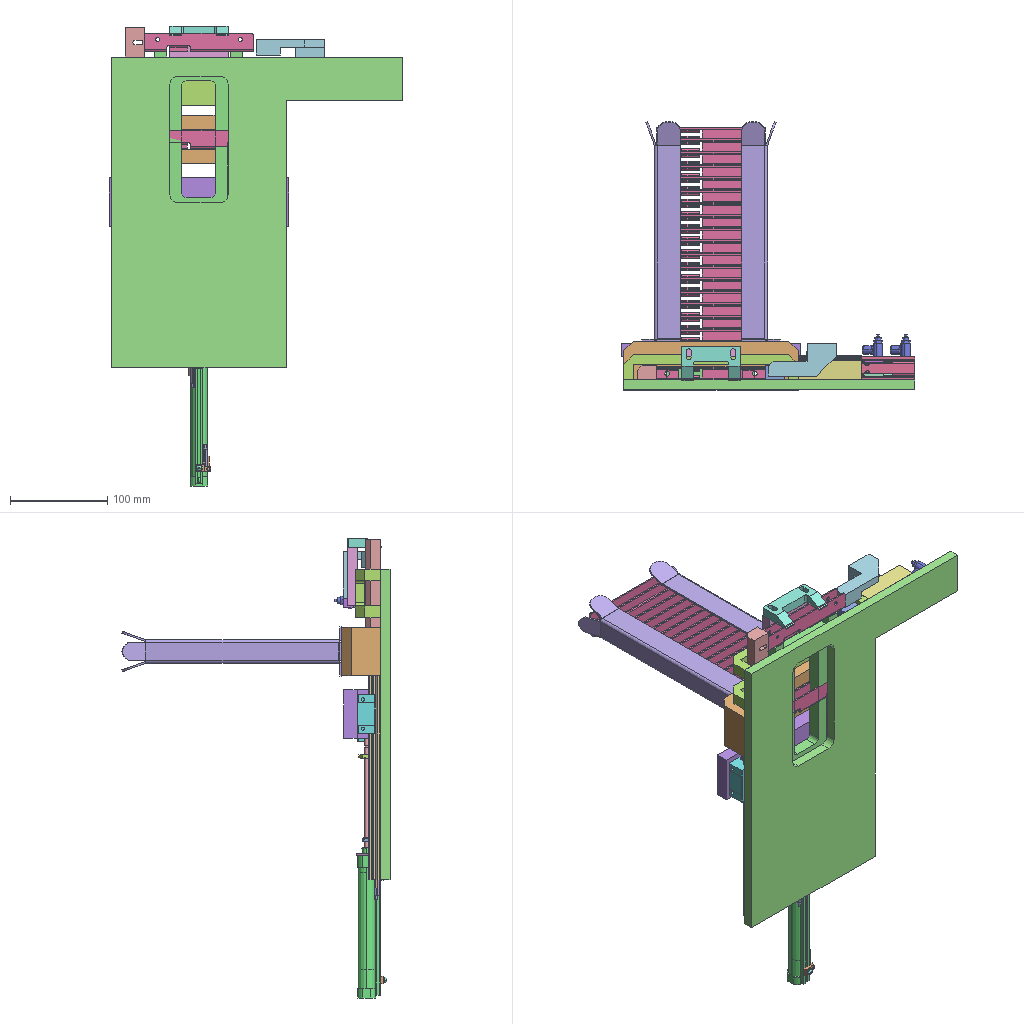Assembly | SolidWorks | 37 different items | 66 placed | box 303 x 276 x 474 mm
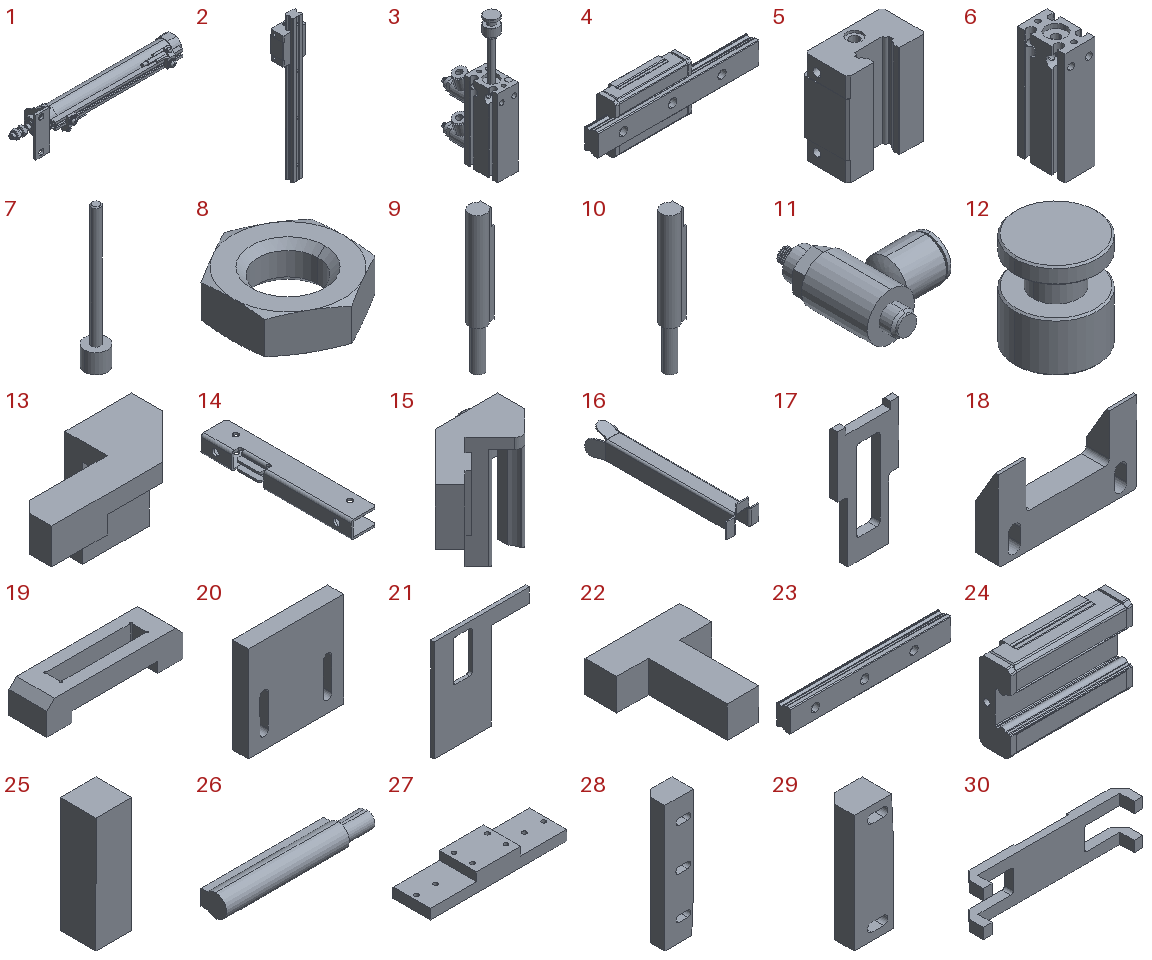Parts list (item | name | quantity | parent item | size | volume | features):
1 | (subassembly) | x1 | - | 175 x 31.65 x 42 mm | 27316 mm3 | -
2 | (subassembly) | x2 | - | 34 x 24 x 210 mm | 54732 mm3 | -
3 | (subassembly) | x1 | - | 16.622 x 46.7 x 96.543 mm | 20146 mm3 | -
4 | (subassembly) | x1 | - | 65 x 10 x 20 mm | 6401 mm3 | -
5 | - | x2 | in 2 | 34 x 19.5 x 40.1 mm | 21289 mm3 | features BaseBody 1
6 | - | x1 | in 3 | 15 x 24 x 56 mm | 13473 mm3 | features BaseBody 1
7 | - | x1 | in 3 | 10 x 10 x 62.6 mm | 1353 mm3 | features BaseBody 1
8 | - | x1 | in 3 | 6 x 6.928 x 2 mm | 44.043 mm3 | features BaseBody 1
9 | - | x1 | in 3 | 4.6 x 4 x 33.5 mm | 397.477 mm3 | features BaseBody 1
10 | - | x1 | in 3 | 4.6 x 4 x 33.5 mm | 397.477 mm3 | features BaseBody 1
11 | - | x2 | in 3 | 20.5 x 26.2 x 10 mm | 1922 mm3 | features BaseBody 1
12 | - | x1 | in 3 | 10 x 10 x 11.5 mm | 637.742 mm3 | features ICE 2, Chamfer 1, Extrusion 1, HoleWzd 1
13 | - | x1 | - | 70 x 34 x 48 mm | 23760 mm3 | features ICE 3, Chamfer 2, Extrusion 1
14 | - | x21 | - | 19 x 112 x 13 mm | 7436 mm3 | features BaseBody 1
15 | - | x2 | in 1 | 15.769 x 11.133 x 16 mm | 523.118 mm3 | features RefAxis 6, ICE 4, 3DProfileFeature 2, Extrusion 1, RevCut 1, Revolution 1
16 | - | x2 | - | 50.5 x 226.176 x 40 mm | 34108 mm3 | features EdgeFlange 3, Fillet 1, FlatPattern 1, SMBaseFlange 1, SheetMetal 1
17 | - | x1 | - | 90 x 12.5 x 180 mm | 108281 mm3 | features Fillet 3, Cut 2, Chamfer 1, Extrusion 1, ICE 1
18 | - | x1 | - | 60 x 10 x 35 mm | 11142 mm3 | features Chamfer 2, Cut 1, Extrusion 1, Fillet 1, ICE 1, MirrorPattern 1
19 | - | x1 | - | 180 x 50 x 40 mm | 216729 mm3 | features ICE 3, Chamfer 1, Cut 1, Extrusion 1
20 | - | x1 | - | 60 x 10 x 60 mm | 33382 mm3 | features Cut 1, Extrusion 1, MirrorPattern 1
21 | - | x1 | - | 300 x 10 x 320 mm | 552549 mm3 | features Cut 1, Extrusion 1, Fillet 1, ICE 1
22 | - | x1 | - | 30 x 35 x 10 mm | 5500 mm3 | features Extrusion 1, ICE 1
23 | - | x1 | in 4 | 65 x 5.5 x 9 mm | 2567 mm3 | features BaseBody 1, Cut 1, HoleWzd 1, ICE 1, LPattern 1
24 | - | x1 | in 4 | 30.8 x 8.5 x 20 mm | 3834 mm3 | features BaseBody 1
25 | - | x1 | - | 20 x 20 x 65 mm | 26000 mm3 | features Extrusion 1
26 | - | x2 | in 1 | 27 x 4.6 x 4 mm | 358.79 mm3 | features RefAxis 3, 3DProfileFeature 1, Extrusion 1, HoleWzd 1, ICE 1
27 | - | x1 | - | 185 x 50 x 25 mm | 153218 mm3 | features HoleWzd 2, Extrusion 1, ICE 1
28 | - | x1 | - | 20 x 15 x 90 mm | 22961 mm3 | features Cut 3, Chamfer 1, Extrusion 1, LPattern 1
29 | - | x1 | - | 20 x 15 x 60 mm | 15035 mm3 | features Cut 3, Chamfer 1, Extrusion 1, MirrorPattern 1
30 | - | x1 | - | 180 x 26 x 50 mm | 63357 mm3 | features Cut 2, Chamfer 1, Extrusion 1, Fillet 1, ICE 1, MirrorPattern 1
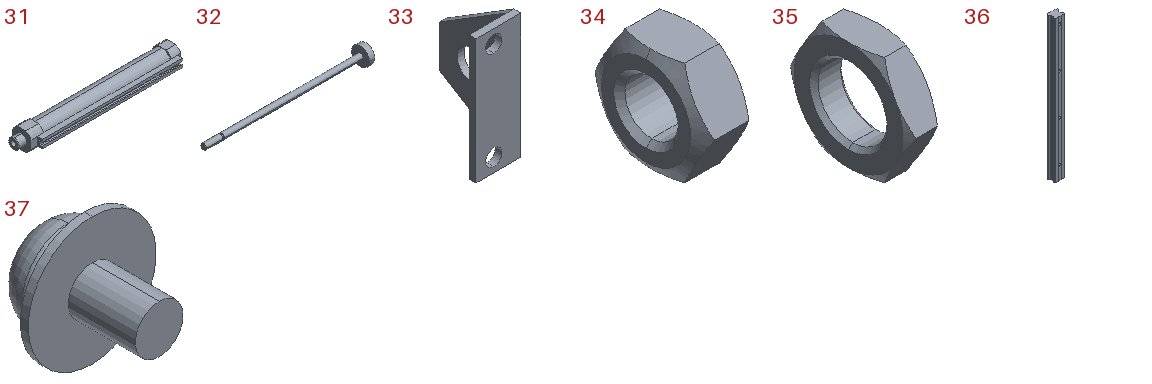31 | - | x1 | in 1 | 155 x 23.3 x 18.3 mm | 18210 mm3 | features RefAxis 21, 3DProfileFeature 7, ICE 4, HoleWzd 2, Revolution 2, LPattern 1, RevCut 1
32 | - | x1 | in 1 | 145.5 x 16 x 16 mm | 3753 mm3 | features RefAxis 9, 3DProfileFeature 3, Revolution 1
33 | - | x1 | in 1 | 15 x 25 x 42 mm | 2621 mm3 | features RefAxis 3, ICE 2, 3DProfileFeature 1, Extrusion 1, HoleWzd 1, LPattern 1
34 | - | x2 | in 1 | 4 x 9.238 x 8 mm | 156.615 mm3 | features RefAxis 6, 3DProfileFeature 2, RevCut 2, Extrusion 1
35 | - | x1 | in 1 | 4 x 16.166 x 14 mm | 414.657 mm3 | features RefAxis 6, 3DProfileFeature 2, RevCut 2, Extrusion 1
36 | - | x2 | in 2 | 15 x 12.5 x 210 mm | 33443 mm3 | features BaseBody 1, HoleWzd 1, ICE 1, LPattern 1
37 | - | x2 | in 1 | 8 x 7.7 x 8 mm | 119.911 mm3 | features RefAxis 6, 3DProfileFeature 2, Revolution 1
Mates (type | each side: item.copy, entity, surface, feature):
In the top assembly
Coincident | 28.1 face plane Boss-Extrude1 | 19.1 face plane Boss-Extrude1
Coincident | 30.1 face plane Cut-Extrude2 | 20.1 face plane Boss-Extrude1 | 2 times
Coincident | 20.1 face plane Boss-Extrude1 | 18.1 face plane Boss-Extrude1 | 2 times
Width | 20.1 face plane Boss-Extrude1 | 20.1 face plane Boss-Extrude1 | 18.1 face plane Boss-Extrude1 | 18.1 face plane Boss-Extrude1
Coincident | 19.1 face plane Boss-Extrude1 | 16.1 face plane Edge-Flange2
Coincident | 19.1 face plane Boss-Extrude1 | 16.2 face plane Edge-Flange2
Width | 19.1 face plane Cut-Extrude3 | 19.1 face plane Cut-Extrude3 | 17.1 face plane Boss-Extrude1 | 17.1 face plane Boss-Extrude1
Coincident | 19.1 face plane Boss-Extrude1 | 36.1 face plane Boss-Extrude1
Coincident | 19.1 face plane Boss-Extrude1 | 36.2 face plane Boss-Extrude1
Coincident | 16.1 face plane Edge-Flange1 | 16.2 face plane Edge-Flange1
Coincident | 17.1 face plane Boss-Extrude1 | 27.1 face plane Boss-Extrude1 | 2 times
Coincident | 5.1 face plane Import1 | 27.1 face plane Cut-Extrude1
Width | 5.1 face plane Import1 | 5.2 face plane Import1 | 27.1 face plane Boss-Extrude1 | 27.1 face plane Boss-Extrude1
Coincident | 21.1 face plane Boss-Extrude1 | 28.1 face plane Boss-Extrude1
DistanceDim | 21.1 face plane Boss-Extrude1 | 28.1 face plane Boss-Extrude1
Coincident | 21.1 face plane Boss-Extrude1 | 29.1 face plane Boss-Extrude1 | 2 times
Coincident | 21.1 face plane Boss-Extrude1 | 30.1 face plane Boss-Extrude2
Width | 21.1 face plane Boss-Extrude1 | 21.1 face plane Boss-Extrude1 | 30.1 face plane Boss-Extrude1 | 30.1 face plane Boss-Extrude1
Coincident | 21.1 face plane Boss-Extrude1 | 30.1 face plane Boss-Extrude1
Coincident | 21.1 face plane Boss-Extrude1 | 19.1 face plane Boss-Extrude1
Width | 19.1 face plane Boss-Extrude1 | 19.1 face plane Boss-Extrude1 | 21.1 face plane Boss-Extrude1 | 21.1 face plane Boss-Extrude1
Coincident | 21.1 face plane Boss-Extrude1 | 5.1 face plane Import1
Coincident | 21.1 face plane Boss-Extrude1 | 36.2 face plane Import1
Coincident | 21.1 face plane Boss-Extrude1 | 5.2 face plane Import1
Coincident | 21.1 face plane Boss-Extrude1 | 33.1 face plane Boss-Extrude1
DistanceDim | 28.1 face plane Boss-Extrude1 | 21.1 face plane Boss-Extrude1
DistanceDim | 18.1 face plane Boss-Extrude1 | 21.1 face plane Boss-Extrude1
DistanceDim | 29.1 face plane Boss-Extrude1 | 21.1 face plane Boss-Extrude1
Width | 16.1 face plane Edge-Flange1 | 16.1 face plane Edge-Flange1 | 19.1 face plane Cut-Extrude1 | 19.1 face plane Cut-Extrude1
DistanceDim | 19.1 face plane Cut-Extrude1 | 16.1 face plane Base-Flange1
Width | 16.2 face plane Edge-Flange1 | 16.2 face plane Edge-Flange1 | 19.1 face plane Cut-Extrude1 | 19.1 face plane Cut-Extrude1
DistanceDim | 16.2 face plane Base-Flange1 | 19.1 face plane Cut-Extrude1
Width | 21.1 face plane Boss-Extrude1 | 21.1 face plane Boss-Extrude1 | 33.1 face plane Boss-Extrude1 | 33.1 face plane Boss-Extrude1
Coincident | 17.1 face plane Boss-Extrude1 | 34.1 face plane Boss-Extrude1
Width | 14.1 face plane Import1 | 14.1 face plane Import1 | 16.2 face plane Edge-Flange1 | 16.2 face plane Edge-Flange1
Width | 16.2 face plane Base-Flange1 | 16.1 face plane Base-Flange1 | 14.1 face plane Import1 | 14.1 face plane Import1
Coincident | 21.1 face plane Boss-Extrude1 | 14.1 face plane Import1
Coincident | 21.1 face plane Boss-Extrude1 | 14.2 face plane Import1
Coincident | 28.1 face plane Boss-Extrude1 | 14.2 face plane Import1
Coincident | 17.1 face plane Boss-Extrude1 | 14.2 face plane Import1
Coincident | 30.1 face plane Boss-Extrude1 | 24.1 face plane Import1
Coincident | 24.1 face plane Import1 | 13.1 face plane Boss-Extrude1
Width | 24.1 face plane Import1 | 24.1 face plane Import1 | 13.1 face plane Boss-Extrude1 | 13.1 face plane Boss-Extrude1
Coincident | 30.1 face plane Boss-Extrude1 | 23.1 face plane Boss-Extrude1
Coincident | 21.1 face plane Boss-Extrude1 | 25.1 face plane Boss-Extrude1 | 2 times
Coincident | 30.1 face plane Boss-Extrude1 | 25.1 face plane Boss-Extrude1
Coincident | 6.1 face plane Import1 | 21.1 face plane Boss-Extrude1
Parallel | 6.1 face plane Import1 | 21.1 face plane Boss-Extrude2
Coincident | 23.1 face plane Import1 | 25.1 face plane Boss-Extrude1
Coincident | 6.1 face plane Import1 | 21.1 face plane Boss-Extrude2
DistanceDim | 6.1 face plane Import1 | 21.1 face plane Boss-Extrude2
Coincident | 13.1 face plane Boss-Extrude1 | 22.1 face plane Boss-Extrude1 | 3 times
DistanceDim | 24.1 face plane Import1 | 13.1 face plane Boss-Extrude1
Coincident | 12.1 face plane Boss-Extrude1 | 22.1 face plane Cut-Extrude1
Width | 27.1 face plane Boss-Extrude1 | 27.1 face plane Boss-Extrude1 | 5.2 face plane Import1 | 5.2 face plane Import1
Coincident | 36.1 face plane Import1 | 21.1 face plane Boss-Extrude1
DistanceDim | 33.1 face plane Boss-Extrude1 | 21.1 face plane Boss-Extrude1
In subassembly 4
DistanceDim | 24.2 face plane Import1 | 23.2 face plane Import1
DistanceDim | 23.2 face plane Import1 | 24.2 face plane Import1
In subassembly 3
LimitDistanceDim | 6.2 face plane Import1 | 7.1 face plane Import1
DistanceDim | 8.1 face plane Import1 | 7.1 face plane Import1
Concentric | 7.1 face cylinder Import1 | 8.1 face cylinder Import1
Concentric | 6.2 face cylinder Import1 | 7.1 face cylinder Import1
Concentric | 7.1 face cylinder Import1 | 12.2 face cylinder Boss-Extrude1
Coincident | 8.1 face plane Import1 | 12.2 face plane Boss-Extrude1
Concentric | 6.2 face cylinder Import1 | 11.1 face cylinder Import1
Coincident | 6.2 face plane Import1 | 11.1 face plane Import1
Concentric | 6.2 face cylinder Import1 | 11.2 face cylinder Import1
Coincident | 6.2 face plane Import1 | 11.2 face plane Import1
In subassembly 2
DistanceDim | 5.3 face plane Import1 | 36.3 face plane Import1
Width | 5.3 face plane Import1 | 5.3 face plane Import1 | 36.3 face plane Import1 | 36.3 face plane Import1
In subassembly 1
Coincident | 31.1 axis | 32.1 axis
PlanarAngleDim | 32.1 plane | 31.1 plane
Coincident | 32.1 axis | 34.2 axis
DistanceDim | 34.3 plane | 32.1 plane
Coincident | 32.1 axis | 34.3 axis
PlanarAngleDim | 34.3 plane | 32.1 plane
Coincident | 31.1 axis | 35.1 axis
PlanarAngleDim | 35.1 plane | 31.1 plane
DistanceDim | 33.2 plane | 31.1 plane
Coincident | 31.1 axis | 33.2 axis
PlanarAngleDim | 33.2 plane | 31.1 plane
DistanceDim | 37.1 plane | 31.1 plane
Coincident | 31.1 axis | 37.1 axis
PlanarAngleDim | 37.1 plane | 31.1 plane
DistanceDim | 15.1 plane | 37.1 plane
Coincident | 37.1 axis | 15.1 axis
PlanarAngleDim | 15.1 plane | 37.1 plane
DistanceDim | 26.1 plane | 15.1 plane
Coincident | 15.1 axis | 26.1 axis
PlanarAngleDim | 26.1 plane | 15.1 plane
DistanceDim | 37.2 plane | 31.1 plane
Coincident | 31.1 axis | 37.2 axis
PlanarAngleDim | 37.2 plane | 31.1 plane
DistanceDim | 15.2 plane | 37.2 plane
Coincident | 37.2 axis | 15.2 axis
PlanarAngleDim | 15.2 plane | 37.2 plane
DistanceDim | 26.2 plane | 15.2 plane
Coincident | 15.2 axis | 26.2 axis
PlanarAngleDim | 26.2 plane | 15.2 plane
LimitDistanceDim | 31.1 face plane Revolve1 | 32.1 face plane Revolve1